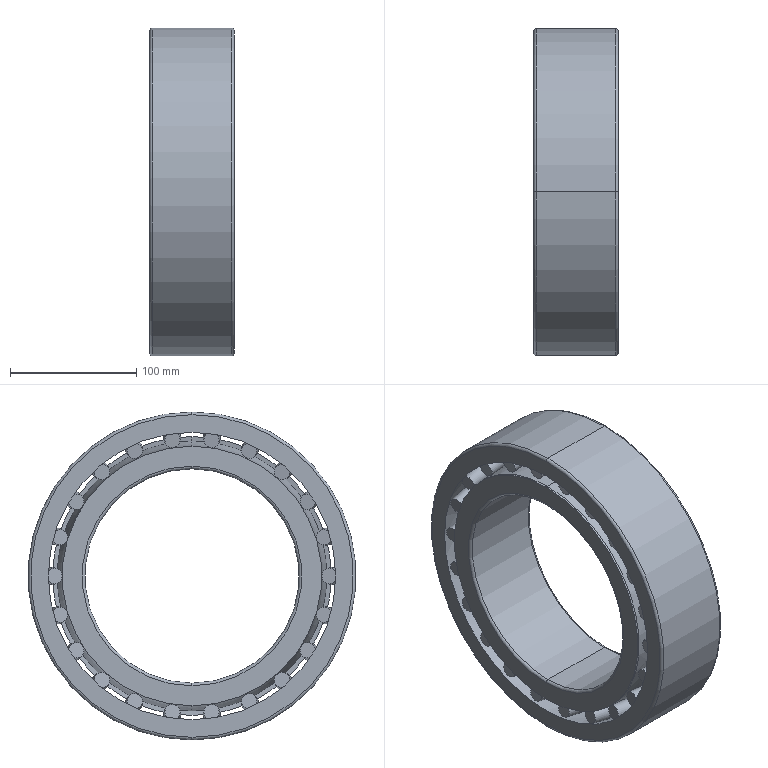Part | SolidWorks | features BaseBody 1 | 1 solid | 250 faces | box 67 x 260 x 260 mm | volume 1601339 mm3 | torus 104 | plane 92 | cone 46 | cylinder 6 | sphere 2 | commonest cylinder face diameters 170 x2 220.625 x2 260 x2